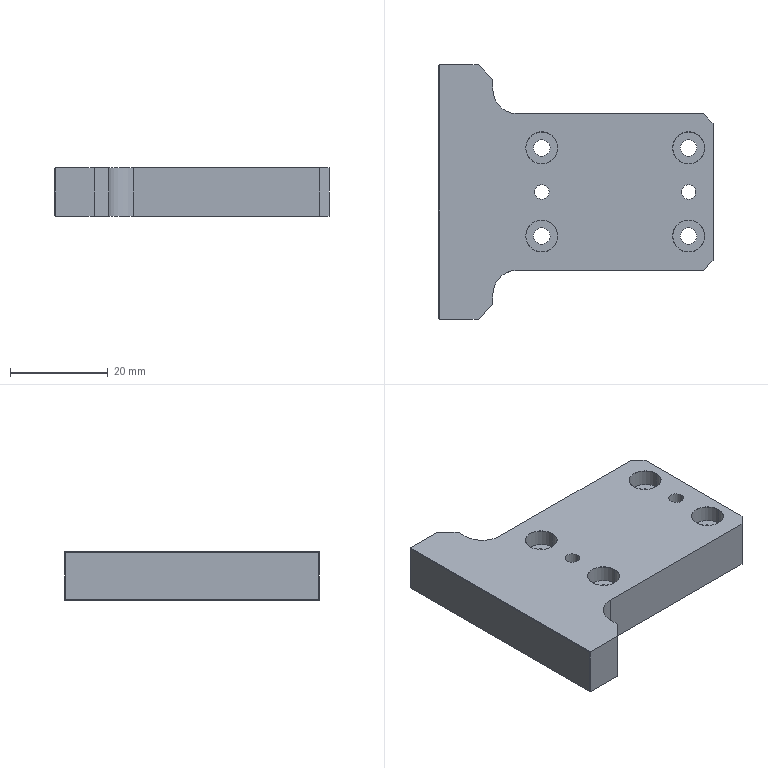Part | STEP file | QA-AD12 | 1 solid | 52 faces | box 56 x 52 x 10 mm | volume 19264 mm3 | cylinder 22 | plane 22 | cone 8 | commonest cylinder face diameters 3.4 x8 6.5 x8 3 x4 10 x2